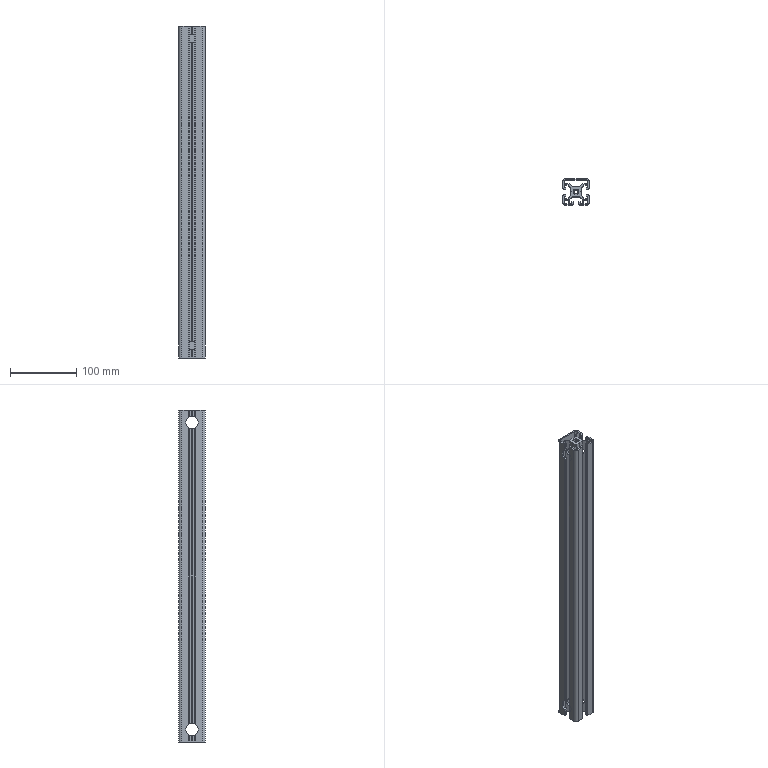Part | SolidWorks | features BaseBody 1, HoleWzd 1, MoveFace 1 | 1 solid | 242 faces | box 40 x 40 x 503 mm | volume 289428 mm3 | plane 187 | cylinder 55 | commonest cylinder face diameters 6.8 x15 2 x14 19 x12 1 x6 5 x4 9 x4